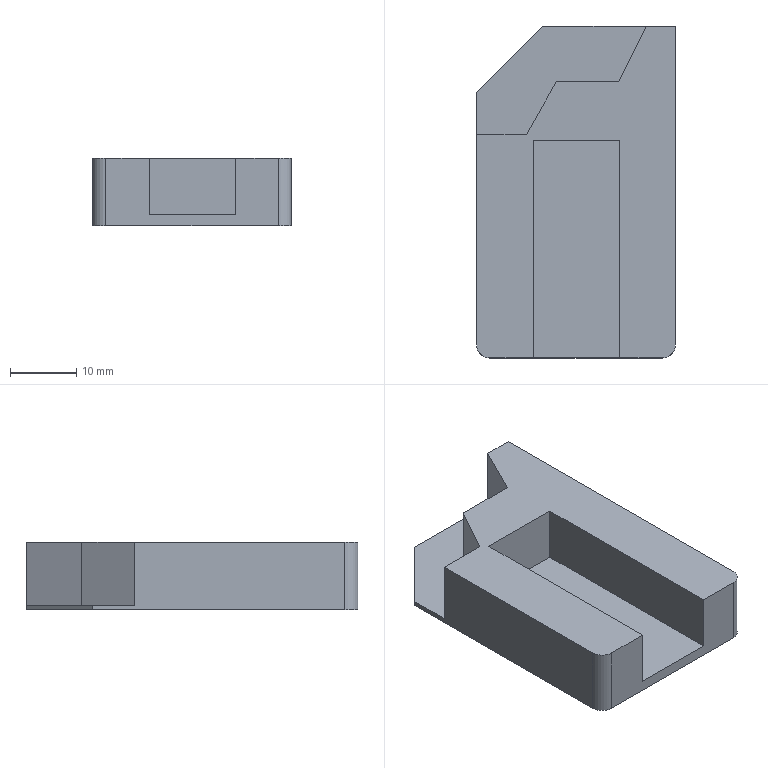Part | SolidWorks | features BaseBody 1 | 1 solid | 18 faces | box 30 x 50 x 10.2 mm | volume 9010 mm3 | plane 16 | cylinder 2 | commonest cylinder face diameters 4 x2
STEP:
#1=CARTESIAN_POINT('',(272.946,-4040.473,2105.871));
#2=VERTEX_POINT('',#1);
#3=CARTESIAN_POINT('',(274.946,-4038.473,2105.871));
#4=VERTEX_POINT('',#3);
#5=CARTESIAN_POINT('',(272.946,-4038.473,2105.871));
#6=DIRECTION('',(0.,0.,1.));
#7=DIRECTION('',(-1.,0.,0.));
#8=AXIS2_PLACEMENT_3D('',#5,#6,#7);
#9=CIRCLE('',#8,2.);
#10=EDGE_CURVE('',#2,#4,#9,.T.);
#11=ORIENTED_EDGE('',*,*,#10,.F.);
#12=CARTESIAN_POINT('',(246.946,-4040.473,2105.871));
#13=VERTEX_POINT('',#12);
#14=CARTESIAN_POINT('',(254.946,-4040.473,2105.871));
#15=DIRECTION('',(1.,0.,0.));
#16=VECTOR('',#15,1000.);
#17=LINE('',#14,#16);
#18=EDGE_CURVE('',#13,#2,#17,.T.);
#19=ORIENTED_EDGE('',*,*,#18,.F.);
#20=CARTESIAN_POINT('',(244.946,-4038.473,2105.871));
#21=VERTEX_POINT('',#20);
#22=CARTESIAN_POINT('',(246.946,-4038.473,2105.871));
#23=DIRECTION('',(0.,0.,1.));
#24=DIRECTION('',(-1.,0.,0.));
#25=AXIS2_PLACEMENT_3D('',#22,#23,#24);
#26=CIRCLE('',#25,2.);
#27=EDGE_CURVE('',#21,#13,#26,.T.);
#28=ORIENTED_EDGE('',*,*,#27,.F.);
#29=CARTESIAN_POINT('',(244.946,-4000.473,2105.871));
#30=VERTEX_POINT('',#29);
#31=CARTESIAN_POINT('',(244.946,-3990.473,2105.871));
#32=DIRECTION('',(0.,-1.,0.));
#33=VECTOR('',#32,1000.);
#34=LINE('',#31,#33);
#35=EDGE_CURVE('',#30,#21,#34,.T.);
#36=ORIENTED_EDGE('',*,*,#35,.F.);
#37=CARTESIAN_POINT('',(254.946,-3990.473,2105.871));
#38=VERTEX_POINT('',#37);
#39=CARTESIAN_POINT('',(254.946,-3990.473,2105.871));
#40=DIRECTION('',(-0.7071,-0.7071,0.));
#41=VECTOR('',#40,1000.);
#42=LINE('',#39,#41);
#43=EDGE_CURVE('',#38,#30,#42,.T.);
#44=ORIENTED_EDGE('',*,*,#43,.F.);
#45=CARTESIAN_POINT('',(274.946,-3990.473,2105.871));
#46=VERTEX_POINT('',#45);
#47=CARTESIAN_POINT('',(254.946,-3990.473,2105.871));
#48=DIRECTION('',(-1.,0.,0.));
#49=VECTOR('',#48,1000.);
#50=LINE('',#47,#49);
#51=EDGE_CURVE('',#46,#38,#50,.T.);
#52=ORIENTED_EDGE('',*,*,#51,.F.);
#53=CARTESIAN_POINT('',(274.946,-3990.473,2105.871));
#54=DIRECTION('',(0.,1.,0.));
#55=VECTOR('',#54,1000.);
#56=LINE('',#53,#55);
#57=EDGE_CURVE('',#4,#46,#56,.T.);
#58=ORIENTED_EDGE('',*,*,#57,.F.);
#59=EDGE_LOOP('',(#11,#19,#28,#36,#44,#52,#58));
#60=FACE_OUTER_BOUND('',#59,.T.);
#61=CARTESIAN_POINT('',(254.946,-3990.473,2105.871));
#62=DIRECTION('',(0.,0.,1.));
#63=DIRECTION('',(0.,-1.,0.));
#64=AXIS2_PLACEMENT_3D('',#61,#62,#63);
#65=PLANE('',#64);
#66=ADVANCED_FACE('',(#60),#65,.F.);
#67=CARTESIAN_POINT('',(274.946,-3990.473,2116.071));
#68=VERTEX_POINT('',#67);
#69=CARTESIAN_POINT('',(274.946,-4038.473,2116.071));
#70=VERTEX_POINT('',#69);
#71=CARTESIAN_POINT('',(274.946,-4025.473,2116.071));
#72=DIRECTION('',(0.,-1.,0.));
#73=VECTOR('',#72,1000.);
#74=LINE('',#71,#73);
#75=EDGE_CURVE('',#68,#70,#74,.T.);
#76=ORIENTED_EDGE('',*,*,#75,.T.);
#77=CARTESIAN_POINT('',(274.946,-4038.473,2106.571));
#78=DIRECTION('',(0.,0.,-1.));
#79=VECTOR('',#78,1000.);
#80=LINE('',#77,#79);
#81=EDGE_CURVE('',#70,#4,#80,.T.);
#82=ORIENTED_EDGE('',*,*,#81,.T.);
#83=ORIENTED_EDGE('',*,*,#57,.T.);
#84=CARTESIAN_POINT('',(274.946,-3990.473,2106.571));
#85=DIRECTION('',(0.,0.,1.));
#86=VECTOR('',#85,1000.);
#87=LINE('',#84,#86);
#88=EDGE_CURVE('',#46,#68,#87,.T.);
#89=ORIENTED_EDGE('',*,*,#88,.T.);
#90=EDGE_LOOP('',(#76,#82,#83,#89));
#91=FACE_OUTER_BOUND('',#90,.T.);
#92=CARTESIAN_POINT('',(274.946,-4025.473,2106.571));
#93=DIRECTION('',(1.,0.,0.));
#94=DIRECTION('',(0.,1.,0.));
#95=AXIS2_PLACEMENT_3D('',#92,#93,#94);
#96=PLANE('',#95);
#97=ADVANCED_FACE('',(#91),#96,.T.);
#98=CARTESIAN_POINT('',(272.946,-4040.473,2116.071));
#99=VERTEX_POINT('',#98);
#100=CARTESIAN_POINT('',(272.946,-4040.473,2106.571));
#101=DIRECTION('',(0.,0.,-1.));
#102=VECTOR('',#101,1000.);
#103=LINE('',#100,#102);
#104=EDGE_CURVE('',#99,#2,#103,.T.);
#105=ORIENTED_EDGE('',*,*,#104,.T.);
#106=ORIENTED_EDGE('',*,*,#10,.T.);
#107=ORIENTED_EDGE('',*,*,#81,.F.);
#108=CARTESIAN_POINT('',(272.946,-4038.473,2116.071));
#109=DIRECTION('',(0.,0.,-1.));
#110=DIRECTION('',(-1.,0.,0.));
#111=AXIS2_PLACEMENT_3D('',#108,#109,#110);
#112=CIRCLE('',#111,2.);
#113=EDGE_CURVE('',#70,#99,#112,.T.);
#114=ORIENTED_EDGE('',*,*,#113,.T.);
#115=EDGE_LOOP('',(#105,#106,#107,#114));
#116=FACE_OUTER_BOUND('',#115,.T.);
#117=CARTESIAN_POINT('',(272.946,-4038.473,2106.571));
#118=DIRECTION('',(0.,0.,-1.));
#119=DIRECTION('',(-1.,0.,0.));
#120=AXIS2_PLACEMENT_3D('',#117,#118,#119);
#121=CYLINDRICAL_SURFACE('',#120,2.);
#122=ADVANCED_FACE('',(#116),#121,.T.);
#123=CARTESIAN_POINT('',(266.541,-4040.473,2116.071));
#124=VERTEX_POINT('',#123);
#125=CARTESIAN_POINT('',(266.541,-4040.473,2107.557));
#126=VERTEX_POINT('',#125);
#127=CARTESIAN_POINT('',(266.541,-4040.473,2106.571));
#128=DIRECTION('',(0.,0.,-1.));
#129=VECTOR('',#128,1000.);
#130=LINE('',#127,#129);
#131=EDGE_CURVE('',#124,#126,#130,.T.);
#132=ORIENTED_EDGE('',*,*,#131,.T.);
#133=CARTESIAN_POINT('',(253.541,-4040.473,2107.557));
#134=VERTEX_POINT('',#133);
#135=CARTESIAN_POINT('',(244.946,-4040.473,2107.557));
#136=DIRECTION('',(-1.,0.,0.));
#137=VECTOR('',#136,1000.);
#138=LINE('',#135,#137);
#139=EDGE_CURVE('',#126,#134,#138,.T.);
#140=ORIENTED_EDGE('',*,*,#139,.T.);
#141=CARTESIAN_POINT('',(253.541,-4040.473,2116.071));
#142=VERTEX_POINT('',#141);
#143=CARTESIAN_POINT('',(253.541,-4040.473,2106.571));
#144=DIRECTION('',(0.,0.,1.));
#145=VECTOR('',#144,1000.);
#146=LINE('',#143,#145);
#147=EDGE_CURVE('',#134,#142,#146,.T.);
#148=ORIENTED_EDGE('',*,*,#147,.T.);
#149=CARTESIAN_POINT('',(246.946,-4040.473,2116.071));
#150=VERTEX_POINT('',#149);
#151=CARTESIAN_POINT('',(244.946,-4040.473,2116.071));
#152=DIRECTION('',(-1.,0.,0.));
#153=VECTOR('',#152,1000.);
#154=LINE('',#151,#153);
#155=EDGE_CURVE('',#142,#150,#154,.T.);
#156=ORIENTED_EDGE('',*,*,#155,.T.);
#157=CARTESIAN_POINT('',(246.946,-4040.473,2106.571));
#158=DIRECTION('',(0.,0.,-1.));
#159=VECTOR('',#158,1000.);
#160=LINE('',#157,#159);
#161=EDGE_CURVE('',#150,#13,#160,.T.);
#162=ORIENTED_EDGE('',*,*,#161,.T.);
#163=ORIENTED_EDGE('',*,*,#18,.T.);
#164=ORIENTED_EDGE('',*,*,#104,.F.);
#165=CARTESIAN_POINT('',(244.946,-4040.473,2116.071));
#166=DIRECTION('',(-1.,0.,0.));
#167=VECTOR('',#166,1000.);
#168=LINE('',#165,#167);
#169=EDGE_CURVE('',#99,#124,#168,.T.);
#170=ORIENTED_EDGE('',*,*,#169,.T.);
#171=EDGE_LOOP('',(#132,#140,#148,#156,#162,#163,#164,#170));
#172=FACE_OUTER_BOUND('',#171,.T.);
#173=CARTESIAN_POINT('',(244.946,-4040.473,2106.571));
#174=DIRECTION('',(0.,-1.,0.));
#175=DIRECTION('',(0.,0.,-1.));
#176=AXIS2_PLACEMENT_3D('',#173,#174,#175);
#177=PLANE('',#176);
#178=ADVANCED_FACE('',(#172),#177,.T.);
#179=CARTESIAN_POINT('',(244.946,-4038.473,2116.071));
#180=VERTEX_POINT('',#179);
#181=CARTESIAN_POINT('',(244.946,-4038.473,2106.571));
#182=DIRECTION('',(0.,0.,-1.));
#183=VECTOR('',#182,1000.);
#184=LINE('',#181,#183);
#185=EDGE_CURVE('',#180,#21,#184,.T.);
#186=ORIENTED_EDGE('',*,*,#185,.T.);
#187=ORIENTED_EDGE('',*,*,#27,.T.);
#188=ORIENTED_EDGE('',*,*,#161,.F.);
#189=CARTESIAN_POINT('',(246.946,-4038.473,2116.071));
#190=DIRECTION('',(0.,0.,-1.));
#191=DIRECTION('',(-1.,0.,0.));
#192=AXIS2_PLACEMENT_3D('',#189,#190,#191);
#193=CIRCLE('',#192,2.);
#194=EDGE_CURVE('',#150,#180,#193,.T.);
#195=ORIENTED_EDGE('',*,*,#194,.T.);
#196=EDGE_LOOP('',(#186,#187,#188,#195));
#197=FACE_OUTER_BOUND('',#196,.T.);
#198=CARTESIAN_POINT('',(246.946,-4038.473,2106.571));
#199=DIRECTION('',(0.,0.,-1.));
#200=DIRECTION('',(-1.,0.,0.));
#201=AXIS2_PLACEMENT_3D('',#198,#199,#200);
#202=CYLINDRICAL_SURFACE('',#201,2.);
#203=ADVANCED_FACE('',(#197),#202,.T.);
#204=CARTESIAN_POINT('',(244.946,-4006.835,2106.571));
#205=VERTEX_POINT('',#204);
#206=CARTESIAN_POINT('',(244.946,-4000.473,2106.571));
#207=VERTEX_POINT('',#206);
#208=CARTESIAN_POINT('',(244.946,-4000.473,2106.571));
#209=DIRECTION('',(0.,1.,0.));
#210=VECTOR('',#209,1000.);
#211=LINE('',#208,#210);
#212=EDGE_CURVE('',#205,#207,#211,.T.);
#213=ORIENTED_EDGE('',*,*,#212,.T.);
#214=CARTESIAN_POINT('',(244.946,-4000.473,2106.571));
#215=DIRECTION('',(0.,0.,-1.));
#216=VECTOR('',#215,1000.);
#217=LINE('',#214,#216);
#218=EDGE_CURVE('',#207,#30,#217,.T.);
#219=ORIENTED_EDGE('',*,*,#218,.T.);
#220=ORIENTED_EDGE('',*,*,#35,.T.);
#221=ORIENTED_EDGE('',*,*,#185,.F.);
#222=CARTESIAN_POINT('',(244.946,-4006.835,2116.071));
#223=VERTEX_POINT('',#222);
#224=CARTESIAN_POINT('',(244.946,-4000.473,2116.071));
#225=DIRECTION('',(0.,1.,0.));
#226=VECTOR('',#225,1000.);
#227=LINE('',#224,#226);
#228=EDGE_CURVE('',#180,#223,#227,.T.);
#229=ORIENTED_EDGE('',*,*,#228,.T.);
#230=CARTESIAN_POINT('',(244.946,-4006.835,2106.571));
#231=DIRECTION('',(0.,0.,-1.));
#232=VECTOR('',#231,1000.);
#233=LINE('',#230,#232);
#234=EDGE_CURVE('',#223,#205,#233,.T.);
#235=ORIENTED_EDGE('',*,*,#234,.T.);
#236=EDGE_LOOP('',(#213,#219,#220,#221,#229,#235));
#237=FACE_OUTER_BOUND('',#236,.T.);
#238=CARTESIAN_POINT('',(244.946,-4000.473,2106.571));
#239=DIRECTION('',(-1.,0.,0.));
#240=DIRECTION('',(0.,-1.,0.));
#241=AXIS2_PLACEMENT_3D('',#238,#239,#240);
#242=PLANE('',#241);
#243=ADVANCED_FACE('',(#237),#242,.T.);
#244=CARTESIAN_POINT('',(254.946,-3990.473,2106.571));
#245=VERTEX_POINT('',#244);
#246=CARTESIAN_POINT('',(254.946,-3990.473,2106.571));
#247=DIRECTION('',(0.7071,0.7071,0.));
#248=VECTOR('',#247,1000.);
#249=LINE('',#246,#248);
#250=EDGE_CURVE('',#207,#245,#249,.T.);
#251=ORIENTED_EDGE('',*,*,#250,.T.);
#252=CARTESIAN_POINT('',(254.946,-3990.473,2106.571));
#253=DIRECTION('',(0.,0.,-1.));
#254=VECTOR('',#253,1000.);
#255=LINE('',#252,#254);
#256=EDGE_CURVE('',#245,#38,#255,.T.);
#257=ORIENTED_EDGE('',*,*,#256,.T.);
#258=ORIENTED_EDGE('',*,*,#43,.T.);
#259=ORIENTED_EDGE('',*,*,#218,.F.);
#260=EDGE_LOOP('',(#251,#257,#258,#259));
#261=FACE_OUTER_BOUND('',#260,.T.);
#262=CARTESIAN_POINT('',(254.946,-3990.473,2106.571));
#263=DIRECTION('',(-0.7071,0.7071,0.));
#264=DIRECTION('',(-0.7071,-0.7071,0.));
#265=AXIS2_PLACEMENT_3D('',#262,#263,#264);
#266=PLANE('',#265);
#267=ADVANCED_FACE('',(#261),#266,.T.);
#268=CARTESIAN_POINT('',(270.521,-3990.473,2116.071));
#269=VERTEX_POINT('',#268);
#270=CARTESIAN_POINT('',(274.946,-3990.473,2116.071));
#271=DIRECTION('',(1.,0.,0.));
#272=VECTOR('',#271,1000.);
#273=LINE('',#270,#272);
#274=EDGE_CURVE('',#269,#68,#273,.T.);
#275=ORIENTED_EDGE('',*,*,#274,.T.);
#276=ORIENTED_EDGE('',*,*,#88,.F.);
#277=ORIENTED_EDGE('',*,*,#51,.T.);
#278=ORIENTED_EDGE('',*,*,#256,.F.);
#279=CARTESIAN_POINT('',(270.521,-3990.473,2106.571));
#280=VERTEX_POINT('',#279);
#281=CARTESIAN_POINT('',(274.946,-3990.473,2106.571));
#282=DIRECTION('',(1.,0.,0.));
#283=VECTOR('',#282,1000.);
#284=LINE('',#281,#283);
#285=EDGE_CURVE('',#245,#280,#284,.T.);
#286=ORIENTED_EDGE('',*,*,#285,.T.);
#287=CARTESIAN_POINT('',(270.521,-3990.473,2106.571));
#288=DIRECTION('',(0.,0.,1.));
#289=VECTOR('',#288,1000.);
#290=LINE('',#287,#289);
#291=EDGE_CURVE('',#280,#269,#290,.T.);
#292=ORIENTED_EDGE('',*,*,#291,.T.);
#293=EDGE_LOOP('',(#275,#276,#277,#278,#286,#292));
#294=FACE_OUTER_BOUND('',#293,.T.);
#295=CARTESIAN_POINT('',(274.946,-3990.473,2106.571));
#296=DIRECTION('',(0.,1.,0.));
#297=DIRECTION('',(0.,0.,1.));
#298=AXIS2_PLACEMENT_3D('',#295,#296,#297);
#299=PLANE('',#298);
#300=ADVANCED_FACE('',(#294),#299,.T.);
#301=ORIENTED_EDGE('',*,*,#194,.F.);
#302=ORIENTED_EDGE('',*,*,#155,.F.);
#303=CARTESIAN_POINT('',(253.541,-4007.733,2116.071));
#304=VERTEX_POINT('',#303);
#305=CARTESIAN_POINT('',(253.541,-4005.41,2116.071));
#306=DIRECTION('',(0.,1.,0.));
#307=VECTOR('',#306,1000.);
#308=LINE('',#305,#307);
#309=EDGE_CURVE('',#142,#304,#308,.T.);
#310=ORIENTED_EDGE('',*,*,#309,.T.);
#311=CARTESIAN_POINT('',(266.541,-4007.733,2116.071));
#312=VERTEX_POINT('',#311);
#313=CARTESIAN_POINT('',(260.766,-4007.733,2116.071));
#314=DIRECTION('',(1.,0.,0.));
#315=VECTOR('',#314,1000.);
#316=LINE('',#313,#315);
#317=EDGE_CURVE('',#304,#312,#316,.T.);
#318=ORIENTED_EDGE('',*,*,#317,.T.);
#319=CARTESIAN_POINT('',(266.541,-4005.41,2116.071));
#320=DIRECTION('',(0.,-1.,0.));
#321=VECTOR('',#320,1000.);
#322=LINE('',#319,#321);
#323=EDGE_CURVE('',#312,#124,#322,.T.);
#324=ORIENTED_EDGE('',*,*,#323,.T.);
#325=ORIENTED_EDGE('',*,*,#169,.F.);
#326=ORIENTED_EDGE('',*,*,#113,.F.);
#327=ORIENTED_EDGE('',*,*,#75,.F.);
#328=ORIENTED_EDGE('',*,*,#274,.F.);
#329=CARTESIAN_POINT('',(266.357,-3998.859,2116.071));
#330=VERTEX_POINT('',#329);
#331=CARTESIAN_POINT('',(270.521,-3990.473,2116.071));
#332=DIRECTION('',(-0.4447,-0.8957,0.));
#333=VECTOR('',#332,1000.);
#334=LINE('',#331,#333);
#335=EDGE_CURVE('',#269,#330,#334,.T.);
#336=ORIENTED_EDGE('',*,*,#335,.T.);
#337=CARTESIAN_POINT('',(256.989,-3998.859,2116.071));
#338=VERTEX_POINT('',#337);
#339=CARTESIAN_POINT('',(260.766,-3998.859,2116.071));
#340=DIRECTION('',(-1.,0.,0.));
#341=VECTOR('',#340,1000.);
#342=LINE('',#339,#341);
#343=EDGE_CURVE('',#330,#338,#342,.T.);
#344=ORIENTED_EDGE('',*,*,#343,.T.);
#345=CARTESIAN_POINT('',(252.478,-4006.835,2116.071));
#346=VERTEX_POINT('',#345);
#347=CARTESIAN_POINT('',(256.989,-3998.859,2116.071));
#348=DIRECTION('',(-0.4923,-0.8704,0.));
#349=VECTOR('',#348,1000.);
#350=LINE('',#347,#349);
#351=EDGE_CURVE('',#338,#346,#350,.T.);
#352=ORIENTED_EDGE('',*,*,#351,.T.);
#353=CARTESIAN_POINT('',(260.766,-4006.835,2116.071));
#354=DIRECTION('',(-1.,0.,0.));
#355=VECTOR('',#354,1000.);
#356=LINE('',#353,#355);
#357=EDGE_CURVE('',#346,#223,#356,.T.);
#358=ORIENTED_EDGE('',*,*,#357,.T.);
#359=ORIENTED_EDGE('',*,*,#228,.F.);
#360=EDGE_LOOP('',(#301,#302,#310,#318,#324,#325,#326,#327,#328,#336,#344,#352,#358,#359));
#361=FACE_OUTER_BOUND('',#360,.T.);
#362=CARTESIAN_POINT('',(260.766,-4005.41,2116.071));
#363=DIRECTION('',(0.,0.,1.));
#364=DIRECTION('',(0.,-1.,0.));
#365=AXIS2_PLACEMENT_3D('',#362,#363,#364);
#366=PLANE('',#365);
#367=ADVANCED_FACE('',(#361),#366,.T.);
#368=CARTESIAN_POINT('',(266.541,-4007.733,2107.557));
#369=VERTEX_POINT('',#368);
#370=CARTESIAN_POINT('',(266.541,-4007.733,2107.557));
#371=DIRECTION('',(0.,-1.,0.));
#372=VECTOR('',#371,1000.);
#373=LINE('',#370,#372);
#374=EDGE_CURVE('',#369,#126,#373,.T.);
#375=ORIENTED_EDGE('',*,*,#374,.F.);
#376=CARTESIAN_POINT('',(253.541,-4007.733,2107.557));
#377=VERTEX_POINT('',#376);
#378=CARTESIAN_POINT('',(266.541,-4007.733,2107.557));
#379=DIRECTION('',(1.,0.,0.));
#380=VECTOR('',#379,1000.);
#381=LINE('',#378,#380);
#382=EDGE_CURVE('',#377,#369,#381,.T.);
#383=ORIENTED_EDGE('',*,*,#382,.F.);
#384=CARTESIAN_POINT('',(253.541,-4007.733,2107.557));
#385=DIRECTION('',(0.,1.,0.));
#386=VECTOR('',#385,1000.);
#387=LINE('',#384,#386);
#388=EDGE_CURVE('',#134,#377,#387,.T.);
#389=ORIENTED_EDGE('',*,*,#388,.F.);
#390=ORIENTED_EDGE('',*,*,#139,.F.);
#391=EDGE_LOOP('',(#375,#383,#389,#390));
#392=FACE_OUTER_BOUND('',#391,.T.);
#393=CARTESIAN_POINT('',(266.541,-4007.733,2107.557));
#394=DIRECTION('',(0.,0.,-1.));
#395=DIRECTION('',(0.,1.,0.));
#396=AXIS2_PLACEMENT_3D('',#393,#394,#395);
#397=PLANE('',#396);
#398=ADVANCED_FACE('',(#392),#397,.F.);
#399=CARTESIAN_POINT('',(266.541,-4007.733,2111.814));
#400=DIRECTION('',(0.,0.,-1.));
#401=VECTOR('',#400,1000.);
#402=LINE('',#399,#401);
#403=EDGE_CURVE('',#312,#369,#402,.T.);
#404=ORIENTED_EDGE('',*,*,#403,.T.);
#405=ORIENTED_EDGE('',*,*,#374,.T.);
#406=ORIENTED_EDGE('',*,*,#131,.F.);
#407=ORIENTED_EDGE('',*,*,#323,.F.);
#408=EDGE_LOOP('',(#404,#405,#406,#407));
#409=FACE_OUTER_BOUND('',#408,.T.);
#410=CARTESIAN_POINT('',(266.541,-4027.305,2111.814));
#411=DIRECTION('',(-1.,0.,0.));
#412=DIRECTION('',(0.,-1.,0.));
#413=AXIS2_PLACEMENT_3D('',#410,#411,#412);
#414=PLANE('',#413);
#415=ADVANCED_FACE('',(#409),#414,.T.);
#416=ORIENTED_EDGE('',*,*,#388,.T.);
#417=CARTESIAN_POINT('',(253.541,-4007.733,2107.557));
#418=DIRECTION('',(0.,0.,-1.));
#419=VECTOR('',#418,1000.);
#420=LINE('',#417,#419);
#421=EDGE_CURVE('',#304,#377,#420,.T.);
#422=ORIENTED_EDGE('',*,*,#421,.F.);
#423=ORIENTED_EDGE('',*,*,#309,.F.);
#424=ORIENTED_EDGE('',*,*,#147,.F.);
#425=EDGE_LOOP('',(#416,#422,#423,#424));
#426=FACE_OUTER_BOUND('',#425,.T.);
#427=CARTESIAN_POINT('',(253.541,-4007.733,2107.557));
#428=DIRECTION('',(-1.,0.,0.));
#429=DIRECTION('',(0.,-1.,0.));
#430=AXIS2_PLACEMENT_3D('',#427,#428,#429);
#431=PLANE('',#430);
#432=ADVANCED_FACE('',(#426),#431,.F.);
#433=ORIENTED_EDGE('',*,*,#250,.F.);
#434=ORIENTED_EDGE('',*,*,#212,.F.);
#435=CARTESIAN_POINT('',(252.478,-4006.835,2106.571));
#436=VERTEX_POINT('',#435);
#437=CARTESIAN_POINT('',(258.946,-4006.835,2106.571));
#438=DIRECTION('',(1.,0.,0.));
#439=VECTOR('',#438,1000.);
#440=LINE('',#437,#439);
#441=EDGE_CURVE('',#205,#436,#440,.T.);
#442=ORIENTED_EDGE('',*,*,#441,.T.);
#443=CARTESIAN_POINT('',(256.989,-3998.859,2106.571));
#444=VERTEX_POINT('',#443);
#445=CARTESIAN_POINT('',(252.478,-4006.835,2106.571));
#446=DIRECTION('',(0.4923,0.8704,0.));
#447=VECTOR('',#446,1000.);
#448=LINE('',#445,#447);
#449=EDGE_CURVE('',#436,#444,#448,.T.);
#450=ORIENTED_EDGE('',*,*,#449,.T.);
#451=CARTESIAN_POINT('',(266.357,-3998.859,2106.571));
#452=VERTEX_POINT('',#451);
#453=CARTESIAN_POINT('',(258.946,-3998.859,2106.571));
#454=DIRECTION('',(1.,0.,0.));
#455=VECTOR('',#454,1000.);
#456=LINE('',#453,#455);
#457=EDGE_CURVE('',#444,#452,#456,.T.);
#458=ORIENTED_EDGE('',*,*,#457,.T.);
#459=CARTESIAN_POINT('',(266.357,-3998.859,2106.571));
#460=DIRECTION('',(0.4447,0.8957,0.));
#461=VECTOR('',#460,1000.);
#462=LINE('',#459,#461);
#463=EDGE_CURVE('',#452,#280,#462,.T.);
#464=ORIENTED_EDGE('',*,*,#463,.T.);
#465=ORIENTED_EDGE('',*,*,#285,.F.);
#466=EDGE_LOOP('',(#433,#434,#442,#450,#458,#464,#465));
#467=FACE_OUTER_BOUND('',#466,.T.);
#468=CARTESIAN_POINT('',(258.946,-4006.473,2106.571));
#469=DIRECTION('',(0.,0.,1.));
#470=DIRECTION('',(0.,-1.,0.));
#471=AXIS2_PLACEMENT_3D('',#468,#469,#470);
#472=PLANE('',#471);
#473=ADVANCED_FACE('',(#467),#472,.T.);
#474=ORIENTED_EDGE('',*,*,#357,.F.);
#475=CARTESIAN_POINT('',(252.478,-4006.835,2116.071));
#476=DIRECTION('',(0.,0.,-1.));
#477=VECTOR('',#476,1000.);
#478=LINE('',#475,#477);
#479=EDGE_CURVE('',#346,#436,#478,.T.);
#480=ORIENTED_EDGE('',*,*,#479,.T.);
#481=ORIENTED_EDGE('',*,*,#441,.F.);
#482=ORIENTED_EDGE('',*,*,#234,.F.);
#483=EDGE_LOOP('',(#474,#480,#481,#482));
#484=FACE_OUTER_BOUND('',#483,.T.);
#485=CARTESIAN_POINT('',(252.478,-4006.835,2116.071));
#486=DIRECTION('',(0.,1.,0.));
#487=DIRECTION('',(0.,0.,1.));
#488=AXIS2_PLACEMENT_3D('',#485,#486,#487);
#489=PLANE('',#488);
#490=ADVANCED_FACE('',(#484),#489,.T.);
#491=ORIENTED_EDGE('',*,*,#335,.F.);
#492=ORIENTED_EDGE('',*,*,#291,.F.);
#493=ORIENTED_EDGE('',*,*,#463,.F.);
#494=CARTESIAN_POINT('',(266.357,-3998.859,2116.071));
#495=DIRECTION('',(0.,0.,1.));
#496=VECTOR('',#495,1000.);
#497=LINE('',#494,#496);
#498=EDGE_CURVE('',#452,#330,#497,.T.);
#499=ORIENTED_EDGE('',*,*,#498,.T.);
#500=EDGE_LOOP('',(#491,#492,#493,#499));
#501=FACE_OUTER_BOUND('',#500,.T.);
#502=CARTESIAN_POINT('',(270.521,-3990.473,2116.071));
#503=DIRECTION('',(-0.8957,0.4447,0.));
#504=DIRECTION('',(-0.4447,-0.8957,0.));
#505=AXIS2_PLACEMENT_3D('',#502,#503,#504);
#506=PLANE('',#505);
#507=ADVANCED_FACE('',(#501),#506,.T.);
#508=ORIENTED_EDGE('',*,*,#351,.F.);
#509=CARTESIAN_POINT('',(256.989,-3998.859,2116.071));
#510=DIRECTION('',(0.,0.,-1.));
#511=VECTOR('',#510,1000.);
#512=LINE('',#509,#511);
#513=EDGE_CURVE('',#338,#444,#512,.T.);
#514=ORIENTED_EDGE('',*,*,#513,.T.);
#515=ORIENTED_EDGE('',*,*,#449,.F.);
#516=ORIENTED_EDGE('',*,*,#479,.F.);
#517=EDGE_LOOP('',(#508,#514,#515,#516));
#518=FACE_OUTER_BOUND('',#517,.T.);
#519=CARTESIAN_POINT('',(256.989,-3998.859,2116.071));
#520=DIRECTION('',(-0.8704,0.4923,0.));
#521=DIRECTION('',(-0.4923,-0.8704,0.));
#522=AXIS2_PLACEMENT_3D('',#519,#520,#521);
#523=PLANE('',#522);
#524=ADVANCED_FACE('',(#518),#523,.T.);
#525=ORIENTED_EDGE('',*,*,#343,.F.);
#526=ORIENTED_EDGE('',*,*,#498,.F.);
#527=ORIENTED_EDGE('',*,*,#457,.F.);
#528=ORIENTED_EDGE('',*,*,#513,.F.);
#529=EDGE_LOOP('',(#525,#526,#527,#528));
#530=FACE_OUTER_BOUND('',#529,.T.);
#531=CARTESIAN_POINT('',(266.357,-3998.859,2116.071));
#532=DIRECTION('',(0.,1.,0.));
#533=DIRECTION('',(0.,0.,1.));
#534=AXIS2_PLACEMENT_3D('',#531,#532,#533);
#535=PLANE('',#534);
#536=ADVANCED_FACE('',(#530),#535,.T.);
#537=ORIENTED_EDGE('',*,*,#382,.T.);
#538=ORIENTED_EDGE('',*,*,#403,.F.);
#539=ORIENTED_EDGE('',*,*,#317,.F.);
#540=ORIENTED_EDGE('',*,*,#421,.T.);
#541=EDGE_LOOP('',(#537,#538,#539,#540));
#542=FACE_OUTER_BOUND('',#541,.T.);
#543=CARTESIAN_POINT('',(266.541,-4007.733,2116.071));
#544=DIRECTION('',(0.,1.,0.));
#545=DIRECTION('',(0.,0.,1.));
#546=AXIS2_PLACEMENT_3D('',#543,#544,#545);
#547=PLANE('',#546);
#548=ADVANCED_FACE('',(#542),#547,.F.);
#549=CLOSED_SHELL('',(#66,#97,#122,#178,#203,#243,#267,#300,#367,#398,#415,#432,#473,#490,#507,#524,#536,#548));
#550=MANIFOLD_SOLID_BREP('',#549);
#551=CARTESIAN_POINT('',(0.,0.,0.));
#552=DIRECTION('',(0.,0.,1.));
#553=DIRECTION('',(1.,0.,0.));
#554=AXIS2_PLACEMENT_3D('',#551,#552,#553);
#555=(LENGTH_UNIT()NAMED_UNIT(*)SI_UNIT(.MILLI.,.METRE.));
#556=UNCERTAINTY_MEASURE_WITH_UNIT(LENGTH_MEASURE(0.00001),#555,'','');
#557=(NAMED_UNIT(*)PLANE_ANGLE_UNIT()SI_UNIT($,.RADIAN.));
#558=(NAMED_UNIT(*)SI_UNIT($,.STERADIAN.)SOLID_ANGLE_UNIT());
#559=(GEOMETRIC_REPRESENTATION_CONTEXT(3)GLOBAL_UNCERTAINTY_ASSIGNED_CONTEXT((#556))GLOBAL_UNIT_ASSIGNED_CONTEXT((#555,#557,#558))REPRESENTATION_CONTEXT('',''));
#560=ADVANCED_BREP_SHAPE_REPRESENTATION('',(#550,#554),#559);